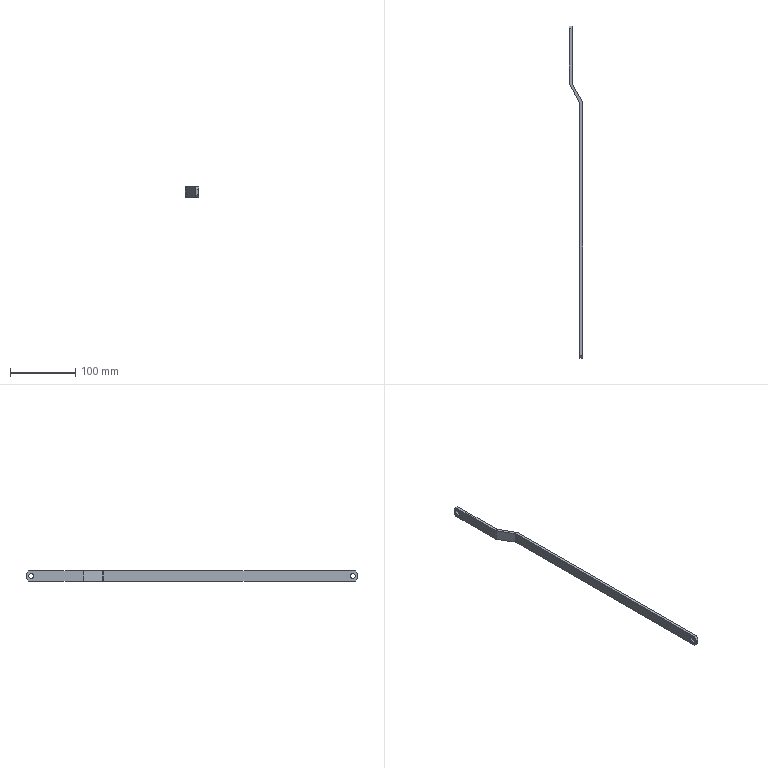Part | STEP file | 8XS174017-2B | 1 solid | 22 faces | box 20 x 510 x 16 mm | volume 32373 mm3 | plane 14 | cylinder 8 | commonest cylinder face diameters 8 x6 16 x2